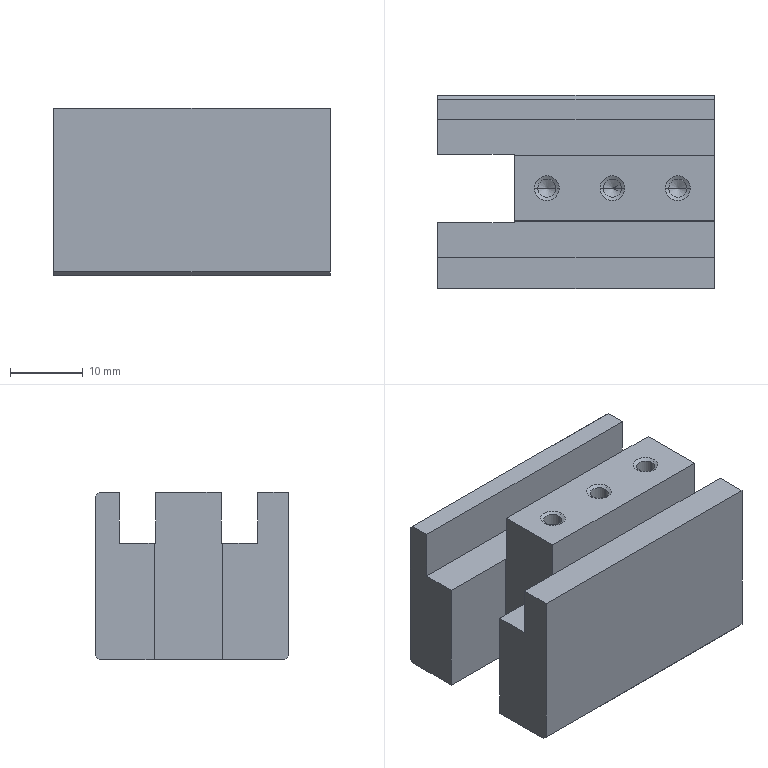Part | NX | 1 solid | 57 faces | box 38 x 26.5 x 22.95 mm | volume 17737 mm3 | cone 24 | plane 21 | cylinder 12 | commonest cylinder face diameters 2.5 x6 3.3 x6
STEP:
#1=CARTESIAN_POINT('',(0.,0.,-22.45));
#2=VERTEX_POINT('',#1);
#3=CARTESIAN_POINT('',(38.,0.,-22.45));
#4=VERTEX_POINT('',#3);
#5=CARTESIAN_POINT('',(0.,0.,-22.45));
#6=DIRECTION('',(1.,0.,0.));
#7=VECTOR('',#6,1000.);
#8=LINE('',#5,#7);
#9=EDGE_CURVE('',#2,#4,#8,.T.);
#10=ORIENTED_EDGE('',*,*,#9,.T.);
#11=CARTESIAN_POINT('',(38.,0.,0.));
#12=VERTEX_POINT('',#11);
#13=CARTESIAN_POINT('',(38.,0.,0.));
#14=DIRECTION('',(0.,0.,-1.));
#15=VECTOR('',#14,1000.);
#16=LINE('',#13,#15);
#17=EDGE_CURVE('',#12,#4,#16,.T.);
#18=ORIENTED_EDGE('',*,*,#17,.F.);
#19=CARTESIAN_POINT('',(0.,0.,0.));
#20=VERTEX_POINT('',#19);
#21=CARTESIAN_POINT('',(0.,0.,0.));
#22=DIRECTION('',(-1.,0.,0.));
#23=VECTOR('',#22,1000.);
#24=LINE('',#21,#23);
#25=EDGE_CURVE('',#12,#20,#24,.T.);
#26=ORIENTED_EDGE('',*,*,#25,.T.);
#27=CARTESIAN_POINT('',(0.,0.,0.));
#28=DIRECTION('',(0.,0.,1.));
#29=VECTOR('',#28,1000.);
#30=LINE('',#27,#29);
#31=EDGE_CURVE('',#2,#20,#30,.T.);
#32=ORIENTED_EDGE('',*,*,#31,.F.);
#33=EDGE_LOOP('',(#10,#18,#26,#32));
#34=FACE_BOUND('',#33,.T.);
#35=CARTESIAN_POINT('',(0.,0.,0.));
#36=DIRECTION('',(0.,1.,0.));
#37=DIRECTION('',(1.,0.,0.));
#38=AXIS2_PLACEMENT_3D('',#35,#36,#37);
#39=PLANE('',#38);
#40=ADVANCED_FACE('',(#34),#39,.F.);
#41=CARTESIAN_POINT('',(0.,4.25,0.));
#42=VERTEX_POINT('',#41);
#43=CARTESIAN_POINT('',(38.,4.25,0.));
#44=VERTEX_POINT('',#43);
#45=CARTESIAN_POINT('',(0.,4.25,0.));
#46=DIRECTION('',(1.,0.,0.));
#47=VECTOR('',#46,1000.);
#48=LINE('',#45,#47);
#49=EDGE_CURVE('',#42,#44,#48,.T.);
#50=ORIENTED_EDGE('',*,*,#49,.F.);
#51=CARTESIAN_POINT('',(0.,0.,0.));
#52=DIRECTION('',(0.,-1.,0.));
#53=VECTOR('',#52,1000.);
#54=LINE('',#51,#53);
#55=EDGE_CURVE('',#42,#20,#54,.T.);
#56=ORIENTED_EDGE('',*,*,#55,.T.);
#57=ORIENTED_EDGE('',*,*,#25,.F.);
#58=CARTESIAN_POINT('',(38.,0.,0.));
#59=DIRECTION('',(0.,1.,0.));
#60=VECTOR('',#59,1000.);
#61=LINE('',#58,#60);
#62=EDGE_CURVE('',#12,#44,#61,.T.);
#63=ORIENTED_EDGE('',*,*,#62,.T.);
#64=EDGE_LOOP('',(#50,#56,#57,#63));
#65=FACE_BOUND('',#64,.T.);
#66=CARTESIAN_POINT('',(0.,0.,0.));
#67=DIRECTION('',(0.,0.,1.));
#68=DIRECTION('',(1.,0.,0.));
#69=AXIS2_PLACEMENT_3D('',#66,#67,#68);
#70=PLANE('',#69);
#71=ADVANCED_FACE('',(#65),#70,.T.);
#72=ORIENTED_EDGE('',*,*,#49,.T.);
#73=CARTESIAN_POINT('',(38.,4.25,-7.));
#74=VERTEX_POINT('',#73);
#75=CARTESIAN_POINT('',(38.,4.25,0.));
#76=DIRECTION('',(0.,0.,1.));
#77=VECTOR('',#76,1000.);
#78=LINE('',#75,#77);
#79=EDGE_CURVE('',#74,#44,#78,.T.);
#80=ORIENTED_EDGE('',*,*,#79,.F.);
#81=CARTESIAN_POINT('',(0.,4.25,-7.));
#82=VERTEX_POINT('',#81);
#83=CARTESIAN_POINT('',(0.,4.25,-7.));
#84=DIRECTION('',(1.,0.,0.));
#85=VECTOR('',#84,1000.);
#86=LINE('',#83,#85);
#87=EDGE_CURVE('',#82,#74,#86,.T.);
#88=ORIENTED_EDGE('',*,*,#87,.F.);
#89=CARTESIAN_POINT('',(0.,4.25,0.));
#90=DIRECTION('',(0.,0.,-1.));
#91=VECTOR('',#90,1000.);
#92=LINE('',#89,#91);
#93=EDGE_CURVE('',#42,#82,#92,.T.);
#94=ORIENTED_EDGE('',*,*,#93,.F.);
#95=EDGE_LOOP('',(#72,#80,#88,#94));
#96=FACE_BOUND('',#95,.T.);
#97=CARTESIAN_POINT('',(0.,4.25,-7.));
#98=DIRECTION('',(0.,-1.,0.));
#99=DIRECTION('',(0.,0.,-1.));
#100=AXIS2_PLACEMENT_3D('',#97,#98,#99);
#101=PLANE('',#100);
#102=ADVANCED_FACE('',(#96),#101,.F.);
#103=CARTESIAN_POINT('',(0.,9.05,-22.95));
#104=VERTEX_POINT('',#103);
#105=CARTESIAN_POINT('',(0.,9.05,-7.));
#106=VERTEX_POINT('',#105);
#107=CARTESIAN_POINT('',(0.,9.05,0.));
#108=DIRECTION('',(0.,0.,1.));
#109=VECTOR('',#108,1000.);
#110=LINE('',#107,#109);
#111=EDGE_CURVE('',#104,#106,#110,.T.);
#112=ORIENTED_EDGE('',*,*,#111,.F.);
#113=CARTESIAN_POINT('',(0.,0.5,-22.95));
#114=VERTEX_POINT('',#113);
#115=CARTESIAN_POINT('',(0.,0.,-22.95));
#116=DIRECTION('',(0.,-1.,0.));
#117=VECTOR('',#116,1000.);
#118=LINE('',#115,#117);
#119=EDGE_CURVE('',#104,#114,#118,.T.);
#120=ORIENTED_EDGE('',*,*,#119,.T.);
#121=CARTESIAN_POINT('',(0.,-22.45,0.));
#122=DIRECTION('',(0.,-0.7071,0.7071));
#123=VECTOR('',#122,1000.);
#124=LINE('',#121,#123);
#125=EDGE_CURVE('',#114,#2,#124,.T.);
#126=ORIENTED_EDGE('',*,*,#125,.T.);
#127=ORIENTED_EDGE('',*,*,#31,.T.);
#128=ORIENTED_EDGE('',*,*,#55,.F.);
#129=ORIENTED_EDGE('',*,*,#93,.T.);
#130=CARTESIAN_POINT('',(0.,0.,-7.));
#131=DIRECTION('',(0.,-1.,0.));
#132=VECTOR('',#131,1000.);
#133=LINE('',#130,#132);
#134=EDGE_CURVE('',#106,#82,#133,.T.);
#135=ORIENTED_EDGE('',*,*,#134,.F.);
#136=EDGE_LOOP('',(#112,#120,#126,#127,#128,#129,#135));
#137=FACE_BOUND('',#136,.T.);
#138=CARTESIAN_POINT('',(0.,0.,-23.));
#139=DIRECTION('',(-1.,0.,0.));
#140=DIRECTION('',(0.,0.,1.));
#141=AXIS2_PLACEMENT_3D('',#138,#139,#140);
#142=PLANE('',#141);
#143=ADVANCED_FACE('',(#137),#142,.T.);
#144=CARTESIAN_POINT('',(10.5,9.05,-22.95));
#145=VERTEX_POINT('',#144);
#146=CARTESIAN_POINT('',(0.,9.05,-22.95));
#147=DIRECTION('',(1.,0.,0.));
#148=VECTOR('',#147,1000.);
#149=LINE('',#146,#148);
#150=EDGE_CURVE('',#104,#145,#149,.T.);
#151=ORIENTED_EDGE('',*,*,#150,.F.);
#152=ORIENTED_EDGE('',*,*,#111,.T.);
#153=CARTESIAN_POINT('',(10.5,9.05,-7.));
#154=VERTEX_POINT('',#153);
#155=CARTESIAN_POINT('',(0.,9.05,-7.));
#156=DIRECTION('',(-1.,0.,0.));
#157=VECTOR('',#156,1000.);
#158=LINE('',#155,#157);
#159=EDGE_CURVE('',#154,#106,#158,.T.);
#160=ORIENTED_EDGE('',*,*,#159,.F.);
#161=CARTESIAN_POINT('',(10.5,9.05,0.));
#162=DIRECTION('',(0.,0.,1.));
#163=VECTOR('',#162,1000.);
#164=LINE('',#161,#163);
#165=EDGE_CURVE('',#145,#154,#164,.T.);
#166=ORIENTED_EDGE('',*,*,#165,.F.);
#167=EDGE_LOOP('',(#151,#152,#160,#166));
#168=FACE_BOUND('',#167,.T.);
#169=CARTESIAN_POINT('',(10.,9.05,-23.));
#170=DIRECTION('',(0.,-1.,0.));
#171=DIRECTION('',(0.,0.,-1.));
#172=AXIS2_PLACEMENT_3D('',#169,#170,#171);
#173=PLANE('',#172);
#174=ADVANCED_FACE('',(#168),#173,.F.);
#175=CARTESIAN_POINT('',(13.75,13.75,-9.));
#176=VERTEX_POINT('',#175);
#177=CARTESIAN_POINT('',(16.25,13.75,-9.));
#178=VERTEX_POINT('',#177);
#179=CARTESIAN_POINT('',(15.,13.75,-9.));
#180=DIRECTION('',(0.,0.,1.));
#181=DIRECTION('',(1.,0.,0.));
#182=AXIS2_PLACEMENT_3D('',#179,#180,#181);
#183=CIRCLE('',#182,1.25);
#184=EDGE_CURVE('',#176,#178,#183,.T.);
#185=ORIENTED_EDGE('',*,*,#184,.T.);
#186=CARTESIAN_POINT('',(15.,13.75,-9.751));
#187=VERTEX_POINT('',#186);
#188=CARTESIAN_POINT('',(16.25,13.75,-9.));
#189=DIRECTION('',(0.8572,0.,0.515));
#190=VECTOR('',#189,1000.);
#191=LINE('',#188,#190);
#192=EDGE_CURVE('',#178,#187,#191,.F.);
#193=ORIENTED_EDGE('',*,*,#192,.T.);
#194=CARTESIAN_POINT('',(13.75,13.75,-9.));
#195=DIRECTION('',(-0.8572,0.,0.515));
#196=VECTOR('',#195,1000.);
#197=LINE('',#194,#196);
#198=EDGE_CURVE('',#176,#187,#197,.F.);
#199=ORIENTED_EDGE('',*,*,#198,.F.);
#200=EDGE_LOOP('',(#185,#193,#199));
#201=FACE_BOUND('',#200,.T.);
#202=CARTESIAN_POINT('',(15.,13.75,-9.));
#203=DIRECTION('',(0.,0.,1.));
#204=DIRECTION('',(1.,0.,0.));
#205=AXIS2_PLACEMENT_3D('',#202,#203,#204);
#206=CONICAL_SURFACE('',#205,1.25,1.03);
#207=ADVANCED_FACE('',(#201),#206,.F.);
#208=CARTESIAN_POINT('',(10.5,18.45,-22.95));
#209=VERTEX_POINT('',#208);
#210=CARTESIAN_POINT('',(0.,18.45,-22.95));
#211=VERTEX_POINT('',#210);
#212=CARTESIAN_POINT('',(0.,18.45,-22.95));
#213=DIRECTION('',(-1.,0.,0.));
#214=VECTOR('',#213,1000.);
#215=LINE('',#212,#214);
#216=EDGE_CURVE('',#209,#211,#215,.T.);
#217=ORIENTED_EDGE('',*,*,#216,.F.);
#218=CARTESIAN_POINT('',(10.5,18.45,-7.));
#219=VERTEX_POINT('',#218);
#220=CARTESIAN_POINT('',(10.5,18.45,0.));
#221=DIRECTION('',(0.,0.,-1.));
#222=VECTOR('',#221,1000.);
#223=LINE('',#220,#222);
#224=EDGE_CURVE('',#219,#209,#223,.T.);
#225=ORIENTED_EDGE('',*,*,#224,.F.);
#226=CARTESIAN_POINT('',(0.,18.45,-7.));
#227=VERTEX_POINT('',#226);
#228=CARTESIAN_POINT('',(0.,18.45,-7.));
#229=DIRECTION('',(1.,0.,0.));
#230=VECTOR('',#229,1000.);
#231=LINE('',#228,#230);
#232=EDGE_CURVE('',#227,#219,#231,.T.);
#233=ORIENTED_EDGE('',*,*,#232,.F.);
#234=CARTESIAN_POINT('',(0.,18.45,0.));
#235=DIRECTION('',(0.,0.,-1.));
#236=VECTOR('',#235,1000.);
#237=LINE('',#234,#236);
#238=EDGE_CURVE('',#227,#211,#237,.T.);
#239=ORIENTED_EDGE('',*,*,#238,.T.);
#240=EDGE_LOOP('',(#217,#225,#233,#239));
#241=FACE_BOUND('',#240,.T.);
#242=CARTESIAN_POINT('',(0.,18.45,-23.));
#243=DIRECTION('',(0.,1.,0.));
#244=DIRECTION('',(1.,0.,0.));
#245=AXIS2_PLACEMENT_3D('',#242,#243,#244);
#246=PLANE('',#245);
#247=ADVANCED_FACE('',(#241),#246,.F.);
#248=ORIENTED_EDGE('',*,*,#238,.F.);
#249=CARTESIAN_POINT('',(0.,23.25,-7.));
#250=VERTEX_POINT('',#249);
#251=CARTESIAN_POINT('',(0.,0.,-7.));
#252=DIRECTION('',(0.,-1.,0.));
#253=VECTOR('',#252,1000.);
#254=LINE('',#251,#253);
#255=EDGE_CURVE('',#250,#227,#254,.T.);
#256=ORIENTED_EDGE('',*,*,#255,.F.);
#257=CARTESIAN_POINT('',(0.,23.25,0.));
#258=VERTEX_POINT('',#257);
#259=CARTESIAN_POINT('',(0.,23.25,0.));
#260=DIRECTION('',(0.,0.,1.));
#261=VECTOR('',#260,1000.);
#262=LINE('',#259,#261);
#263=EDGE_CURVE('',#250,#258,#262,.T.);
#264=ORIENTED_EDGE('',*,*,#263,.T.);
#265=CARTESIAN_POINT('',(0.,26.,0.));
#266=VERTEX_POINT('',#265);
#267=CARTESIAN_POINT('',(0.,0.,0.));
#268=DIRECTION('',(0.,-1.,0.));
#269=VECTOR('',#268,1000.);
#270=LINE('',#267,#269);
#271=EDGE_CURVE('',#266,#258,#270,.T.);
#272=ORIENTED_EDGE('',*,*,#271,.F.);
#273=CARTESIAN_POINT('',(0.,26.5,-0.5));
#274=VERTEX_POINT('',#273);
#275=CARTESIAN_POINT('',(0.,26.,0.));
#276=DIRECTION('',(0.,0.7071,-0.7071));
#277=VECTOR('',#276,1000.);
#278=LINE('',#275,#277);
#279=EDGE_CURVE('',#266,#274,#278,.T.);
#280=ORIENTED_EDGE('',*,*,#279,.T.);
#281=CARTESIAN_POINT('',(0.,26.5,-22.45));
#282=VERTEX_POINT('',#281);
#283=CARTESIAN_POINT('',(0.,26.5,0.));
#284=DIRECTION('',(0.,0.,1.));
#285=VECTOR('',#284,1000.);
#286=LINE('',#283,#285);
#287=EDGE_CURVE('',#282,#274,#286,.T.);
#288=ORIENTED_EDGE('',*,*,#287,.F.);
#289=CARTESIAN_POINT('',(0.,26.,-22.95));
#290=VERTEX_POINT('',#289);
#291=CARTESIAN_POINT('',(0.,48.95,0.));
#292=DIRECTION('',(0.,-0.7071,-0.7071));
#293=VECTOR('',#292,1000.);
#294=LINE('',#291,#293);
#295=EDGE_CURVE('',#282,#290,#294,.T.);
#296=ORIENTED_EDGE('',*,*,#295,.T.);
#297=CARTESIAN_POINT('',(0.,0.,-22.95));
#298=DIRECTION('',(0.,-1.,0.));
#299=VECTOR('',#298,1000.);
#300=LINE('',#297,#299);
#301=EDGE_CURVE('',#290,#211,#300,.T.);
#302=ORIENTED_EDGE('',*,*,#301,.T.);
#303=EDGE_LOOP('',(#248,#256,#264,#272,#280,#288,#296,#302));
#304=FACE_BOUND('',#303,.T.);
#305=CARTESIAN_POINT('',(0.,0.,-23.));
#306=DIRECTION('',(-1.,0.,0.));
#307=DIRECTION('',(0.,0.,1.));
#308=AXIS2_PLACEMENT_3D('',#305,#306,#307);
#309=PLANE('',#308);
#310=ADVANCED_FACE('',(#304),#309,.T.);
#311=CARTESIAN_POINT('',(38.,26.5,-0.5));
#312=VERTEX_POINT('',#311);
#313=CARTESIAN_POINT('',(0.,26.5,-0.5));
#314=DIRECTION('',(1.,0.,0.));
#315=VECTOR('',#314,1000.);
#316=LINE('',#313,#315);
#317=EDGE_CURVE('',#274,#312,#316,.T.);
#318=ORIENTED_EDGE('',*,*,#317,.T.);
#319=CARTESIAN_POINT('',(38.,26.5,-22.45));
#320=VERTEX_POINT('',#319);
#321=CARTESIAN_POINT('',(38.,26.5,0.));
#322=DIRECTION('',(0.,0.,1.));
#323=VECTOR('',#322,1000.);
#324=LINE('',#321,#323);
#325=EDGE_CURVE('',#320,#312,#324,.T.);
#326=ORIENTED_EDGE('',*,*,#325,.F.);
#327=CARTESIAN_POINT('',(0.,26.5,-22.45));
#328=DIRECTION('',(-1.,0.,0.));
#329=VECTOR('',#328,1000.);
#330=LINE('',#327,#329);
#331=EDGE_CURVE('',#320,#282,#330,.T.);
#332=ORIENTED_EDGE('',*,*,#331,.T.);
#333=ORIENTED_EDGE('',*,*,#287,.T.);
#334=EDGE_LOOP('',(#318,#326,#332,#333));
#335=FACE_BOUND('',#334,.T.);
#336=CARTESIAN_POINT('',(0.,26.5,0.));
#337=DIRECTION('',(0.,1.,0.));
#338=DIRECTION('',(1.,0.,0.));
#339=AXIS2_PLACEMENT_3D('',#336,#337,#338);
#340=PLANE('',#339);
#341=ADVANCED_FACE('',(#335),#340,.T.);
#342=CARTESIAN_POINT('',(38.,23.25,0.));
#343=VERTEX_POINT('',#342);
#344=CARTESIAN_POINT('',(0.,23.25,0.));
#345=DIRECTION('',(-1.,0.,0.));
#346=VECTOR('',#345,1000.);
#347=LINE('',#344,#346);
#348=EDGE_CURVE('',#343,#258,#347,.T.);
#349=ORIENTED_EDGE('',*,*,#348,.F.);
#350=CARTESIAN_POINT('',(38.,26.,0.));
#351=VERTEX_POINT('',#350);
#352=CARTESIAN_POINT('',(38.,0.,0.));
#353=DIRECTION('',(0.,1.,0.));
#354=VECTOR('',#353,1000.);
#355=LINE('',#352,#354);
#356=EDGE_CURVE('',#343,#351,#355,.T.);
#357=ORIENTED_EDGE('',*,*,#356,.T.);
#358=CARTESIAN_POINT('',(0.,26.,0.));
#359=DIRECTION('',(-1.,0.,0.));
#360=VECTOR('',#359,1000.);
#361=LINE('',#358,#360);
#362=EDGE_CURVE('',#351,#266,#361,.T.);
#363=ORIENTED_EDGE('',*,*,#362,.T.);
#364=ORIENTED_EDGE('',*,*,#271,.T.);
#365=EDGE_LOOP('',(#349,#357,#363,#364));
#366=FACE_BOUND('',#365,.T.);
#367=CARTESIAN_POINT('',(0.,0.,0.));
#368=DIRECTION('',(0.,0.,1.));
#369=DIRECTION('',(1.,0.,0.));
#370=AXIS2_PLACEMENT_3D('',#367,#368,#369);
#371=PLANE('',#370);
#372=ADVANCED_FACE('',(#366),#371,.T.);
#373=ORIENTED_EDGE('',*,*,#348,.T.);
#374=ORIENTED_EDGE('',*,*,#263,.F.);
#375=CARTESIAN_POINT('',(38.,23.25,-7.));
#376=VERTEX_POINT('',#375);
#377=CARTESIAN_POINT('',(0.,23.25,-7.));
#378=DIRECTION('',(-1.,0.,0.));
#379=VECTOR('',#378,1000.);
#380=LINE('',#377,#379);
#381=EDGE_CURVE('',#376,#250,#380,.T.);
#382=ORIENTED_EDGE('',*,*,#381,.F.);
#383=CARTESIAN_POINT('',(38.,23.25,0.));
#384=DIRECTION('',(0.,0.,-1.));
#385=VECTOR('',#384,1000.);
#386=LINE('',#383,#385);
#387=EDGE_CURVE('',#343,#376,#386,.T.);
#388=ORIENTED_EDGE('',*,*,#387,.F.);
#389=EDGE_LOOP('',(#373,#374,#382,#388));
#390=FACE_BOUND('',#389,.T.);
#391=CARTESIAN_POINT('',(0.,23.25,0.));
#392=DIRECTION('',(0.,1.,0.));
#393=DIRECTION('',(1.,0.,0.));
#394=AXIS2_PLACEMENT_3D('',#391,#392,#393);
#395=PLANE('',#394);
#396=ADVANCED_FACE('',(#390),#395,.F.);
#397=ORIENTED_EDGE('',*,*,#387,.T.);
#398=CARTESIAN_POINT('',(38.,18.25,-7.));
#399=VERTEX_POINT('',#398);
#400=CARTESIAN_POINT('',(38.,0.,-7.));
#401=DIRECTION('',(0.,1.,0.));
#402=VECTOR('',#401,1000.);
#403=LINE('',#400,#402);
#404=EDGE_CURVE('',#399,#376,#403,.T.);
#405=ORIENTED_EDGE('',*,*,#404,.F.);
#406=CARTESIAN_POINT('',(38.,18.25,0.));
#407=VERTEX_POINT('',#406);
#408=CARTESIAN_POINT('',(38.,18.25,0.));
#409=DIRECTION('',(0.,0.,-1.));
#410=VECTOR('',#409,1000.);
#411=LINE('',#408,#410);
#412=EDGE_CURVE('',#407,#399,#411,.T.);
#413=ORIENTED_EDGE('',*,*,#412,.F.);
#414=CARTESIAN_POINT('',(38.,9.25,0.));
#415=VERTEX_POINT('',#414);
#416=CARTESIAN_POINT('',(38.,0.,0.));
#417=DIRECTION('',(0.,-1.,0.));
#418=VECTOR('',#417,1000.);
#419=LINE('',#416,#418);
#420=EDGE_CURVE('',#407,#415,#419,.T.);
#421=ORIENTED_EDGE('',*,*,#420,.T.);
#422=CARTESIAN_POINT('',(38.,9.25,-7.));
#423=VERTEX_POINT('',#422);
#424=CARTESIAN_POINT('',(38.,9.25,0.));
#425=DIRECTION('',(0.,0.,1.));
#426=VECTOR('',#425,1000.);
#427=LINE('',#424,#426);
#428=EDGE_CURVE('',#423,#415,#427,.T.);
#429=ORIENTED_EDGE('',*,*,#428,.F.);
#430=CARTESIAN_POINT('',(38.,0.,-7.));
#431=DIRECTION('',(0.,1.,0.));
#432=VECTOR('',#431,1000.);
#433=LINE('',#430,#432);
#434=EDGE_CURVE('',#74,#423,#433,.T.);
#435=ORIENTED_EDGE('',*,*,#434,.F.);
#436=ORIENTED_EDGE('',*,*,#79,.T.);
#437=ORIENTED_EDGE('',*,*,#62,.F.);
#438=ORIENTED_EDGE('',*,*,#17,.T.);
#439=CARTESIAN_POINT('',(38.,0.5,-22.95));
#440=VERTEX_POINT('',#439);
#441=CARTESIAN_POINT('',(38.,-22.45,0.));
#442=DIRECTION('',(0.,-0.7071,0.7071));
#443=VECTOR('',#442,1000.);
#444=LINE('',#441,#443);
#445=EDGE_CURVE('',#440,#4,#444,.T.);
#446=ORIENTED_EDGE('',*,*,#445,.F.);
#447=CARTESIAN_POINT('',(38.,26.,-22.95));
#448=VERTEX_POINT('',#447);
#449=CARTESIAN_POINT('',(38.,0.,-22.95));
#450=DIRECTION('',(0.,1.,0.));
#451=VECTOR('',#450,1000.);
#452=LINE('',#449,#451);
#453=EDGE_CURVE('',#440,#448,#452,.T.);
#454=ORIENTED_EDGE('',*,*,#453,.T.);
#455=CARTESIAN_POINT('',(38.,48.95,0.));
#456=DIRECTION('',(0.,-0.7071,-0.7071));
#457=VECTOR('',#456,1000.);
#458=LINE('',#455,#457);
#459=EDGE_CURVE('',#320,#448,#458,.T.);
#460=ORIENTED_EDGE('',*,*,#459,.F.);
#461=ORIENTED_EDGE('',*,*,#325,.T.);
#462=CARTESIAN_POINT('',(38.,26.,0.));
#463=DIRECTION('',(0.,-0.7071,0.7071));
#464=VECTOR('',#463,1000.);
#465=LINE('',#462,#464);
#466=EDGE_CURVE('',#312,#351,#465,.T.);
#467=ORIENTED_EDGE('',*,*,#466,.T.);
#468=ORIENTED_EDGE('',*,*,#356,.F.);
#469=EDGE_LOOP('',(#397,#405,#413,#421,#429,#435,#436,#437,#438,#446,#454,#460,#461,#467,#468));
#470=FACE_BOUND('',#469,.T.);
#471=CARTESIAN_POINT('',(38.,0.,0.));
#472=DIRECTION('',(1.,0.,0.));
#473=DIRECTION('',(0.,1.,0.));
#474=AXIS2_PLACEMENT_3D('',#471,#472,#473);
#475=PLANE('',#474);
#476=ADVANCED_FACE('',(#470),#475,.T.);
#477=CARTESIAN_POINT('',(10.5,9.25,-7.));
#478=VERTEX_POINT('',#477);
#479=CARTESIAN_POINT('',(10.5,0.,-7.));
#480=DIRECTION('',(0.,-1.,0.));
#481=VECTOR('',#480,1000.);
#482=LINE('',#479,#481);
#483=EDGE_CURVE('',#478,#154,#482,.T.);
#484=ORIENTED_EDGE('',*,*,#483,.T.);
#485=ORIENTED_EDGE('',*,*,#159,.T.);
#486=ORIENTED_EDGE('',*,*,#134,.T.);
#487=ORIENTED_EDGE('',*,*,#87,.T.);
#488=ORIENTED_EDGE('',*,*,#434,.T.);
#489=CARTESIAN_POINT('',(0.,9.25,-7.));
#490=DIRECTION('',(1.,0.,0.));
#491=VECTOR('',#490,1000.);
#492=LINE('',#489,#491);
#493=EDGE_CURVE('',#478,#423,#492,.T.);
#494=ORIENTED_EDGE('',*,*,#493,.F.);
#495=EDGE_LOOP('',(#484,#485,#486,#487,#488,#494));
#496=FACE_BOUND('',#495,.T.);
#497=CARTESIAN_POINT('',(0.,9.25,-7.));
#498=DIRECTION('',(0.,0.,-1.));
#499=DIRECTION('',(0.,-1.,0.));
#500=AXIS2_PLACEMENT_3D('',#497,#498,#499);
#501=PLANE('',#500);
#502=ADVANCED_FACE('',(#496),#501,.F.);
#503=CARTESIAN_POINT('',(10.5,18.25,0.));
#504=VERTEX_POINT('',#503);
#505=CARTESIAN_POINT('',(10.5,9.25,0.));
#506=VERTEX_POINT('',#505);
#507=CARTESIAN_POINT('',(10.5,0.,0.));
#508=DIRECTION('',(0.,-1.,0.));
#509=VECTOR('',#508,1000.);
#510=LINE('',#507,#509);
#511=EDGE_CURVE('',#504,#506,#510,.T.);
#512=ORIENTED_EDGE('',*,*,#511,.F.);
#513=CARTESIAN_POINT('',(10.5,18.25,-7.));
#514=VERTEX_POINT('',#513);
#515=CARTESIAN_POINT('',(10.5,18.25,0.));
#516=DIRECTION('',(0.,0.,1.));
#517=VECTOR('',#516,1000.);
#518=LINE('',#515,#517);
#519=EDGE_CURVE('',#514,#504,#518,.T.);
#520=ORIENTED_EDGE('',*,*,#519,.F.);
#521=CARTESIAN_POINT('',(10.5,0.,-7.));
#522=DIRECTION('',(0.,-1.,0.));
#523=VECTOR('',#522,1000.);
#524=LINE('',#521,#523);
#525=EDGE_CURVE('',#219,#514,#524,.T.);
#526=ORIENTED_EDGE('',*,*,#525,.F.);
#527=ORIENTED_EDGE('',*,*,#224,.T.);
#528=CARTESIAN_POINT('',(10.5,0.,-22.95));
#529=DIRECTION('',(0.,1.,0.));
#530=VECTOR('',#529,1000.);
#531=LINE('',#528,#530);
#532=EDGE_CURVE('',#145,#209,#531,.T.);
#533=ORIENTED_EDGE('',*,*,#532,.F.);
#534=ORIENTED_EDGE('',*,*,#165,.T.);
#535=ORIENTED_EDGE('',*,*,#483,.F.);
#536=CARTESIAN_POINT('',(10.5,9.25,0.));
#537=DIRECTION('',(0.,0.,-1.));
#538=VECTOR('',#537,1000.);
#539=LINE('',#536,#538);
#540=EDGE_CURVE('',#506,#478,#539,.T.);
#541=ORIENTED_EDGE('',*,*,#540,.F.);
#542=EDGE_LOOP('',(#512,#520,#526,#527,#533,#534,#535,#541));
#543=FACE_BOUND('',#542,.T.);
#544=CARTESIAN_POINT('',(10.5,18.45,-23.));
#545=DIRECTION('',(1.,0.,0.));
#546=DIRECTION('',(0.,1.,0.));
#547=AXIS2_PLACEMENT_3D('',#544,#545,#546);
#548=PLANE('',#547);
#549=ADVANCED_FACE('',(#543),#548,.F.);
#550=CARTESIAN_POINT('',(0.,26.,-22.95));
#551=DIRECTION('',(1.,0.,0.));
#552=VECTOR('',#551,1000.);
#553=LINE('',#550,#552);
#554=EDGE_CURVE('',#290,#448,#553,.T.);
#555=ORIENTED_EDGE('',*,*,#554,.T.);
#556=ORIENTED_EDGE('',*,*,#453,.F.);
#557=CARTESIAN_POINT('',(0.,0.5,-22.95));
#558=DIRECTION('',(-1.,0.,0.));
#559=VECTOR('',#558,1000.);
#560=LINE('',#557,#559);
#561=EDGE_CURVE('',#440,#114,#560,.T.);
#562=ORIENTED_EDGE('',*,*,#561,.T.);
#563=ORIENTED_EDGE('',*,*,#119,.F.);
#564=ORIENTED_EDGE('',*,*,#150,.T.);
#565=ORIENTED_EDGE('',*,*,#532,.T.);
#566=ORIENTED_EDGE('',*,*,#216,.T.);
#567=ORIENTED_EDGE('',*,*,#301,.F.);
#568=EDGE_LOOP('',(#555,#556,#562,#563,#564,#565,#566,#567));
#569=FACE_BOUND('',#568,.T.);
#570=CARTESIAN_POINT('',(30.685,21.75,-22.95));
#571=VERTEX_POINT('',#570);
#572=CARTESIAN_POINT('',(35.315,21.75,-22.95));
#573=VERTEX_POINT('',#572);
#574=CARTESIAN_POINT('',(33.,21.75,-22.95));
#575=DIRECTION('',(0.,0.,-1.));
#576=DIRECTION('',(-1.,0.,0.));
#577=AXIS2_PLACEMENT_3D('',#574,#575,#576);
#578=CIRCLE('',#577,2.315);
#579=EDGE_CURVE('',#571,#573,#578,.T.);
#580=ORIENTED_EDGE('',*,*,#579,.F.);
#581=CARTESIAN_POINT('',(33.,21.75,-22.95));
#582=DIRECTION('',(0.,0.,-1.));
#583=DIRECTION('',(-1.,0.,0.));
#584=AXIS2_PLACEMENT_3D('',#581,#582,#583);
#585=CIRCLE('',#584,2.315);
#586=EDGE_CURVE('',#573,#571,#585,.T.);
#587=ORIENTED_EDGE('',*,*,#586,.F.);
#588=EDGE_LOOP('',(#580,#587));
#589=FACE_BOUND('',#588,.T.);
#590=CARTESIAN_POINT('',(7.315,21.75,-22.95));
#591=VERTEX_POINT('',#590);
#592=CARTESIAN_POINT('',(2.685,21.75,-22.95));
#593=VERTEX_POINT('',#592);
#594=CARTESIAN_POINT('',(5.,21.75,-22.95));
#595=DIRECTION('',(0.,0.,-1.));
#596=DIRECTION('',(-1.,0.,0.));
#597=AXIS2_PLACEMENT_3D('',#594,#595,#596);
#598=CIRCLE('',#597,2.315);
#599=EDGE_CURVE('',#591,#593,#598,.T.);
#600=ORIENTED_EDGE('',*,*,#599,.F.);
#601=CARTESIAN_POINT('',(5.,21.75,-22.95));
#602=DIRECTION('',(0.,0.,-1.));
#603=DIRECTION('',(-1.,0.,0.));
#604=AXIS2_PLACEMENT_3D('',#601,#602,#603);
#605=CIRCLE('',#604,2.315);
#606=EDGE_CURVE('',#593,#591,#605,.T.);
#607=ORIENTED_EDGE('',*,*,#606,.F.);
#608=EDGE_LOOP('',(#600,#607));
#609=FACE_BOUND('',#608,.T.);
#610=CARTESIAN_POINT('',(16.685,21.75,-22.95));
#611=VERTEX_POINT('',#610);
#612=CARTESIAN_POINT('',(21.315,21.75,-22.95));
#613=VERTEX_POINT('',#612);
#614=CARTESIAN_POINT('',(19.,21.75,-22.95));
#615=DIRECTION('',(0.,0.,-1.));
#616=DIRECTION('',(-1.,0.,0.));
#617=AXIS2_PLACEMENT_3D('',#614,#615,#616);
#618=CIRCLE('',#617,2.315);
#619=EDGE_CURVE('',#611,#613,#618,.T.);
#620=ORIENTED_EDGE('',*,*,#619,.F.);
#621=CARTESIAN_POINT('',(19.,21.75,-22.95));
#622=DIRECTION('',(0.,0.,-1.));
#623=DIRECTION('',(-1.,0.,0.));
#624=AXIS2_PLACEMENT_3D('',#621,#622,#623);
#625=CIRCLE('',#624,2.315);
#626=EDGE_CURVE('',#613,#611,#625,.T.);
#627=ORIENTED_EDGE('',*,*,#626,.F.);
#628=EDGE_LOOP('',(#620,#627));
#629=FACE_BOUND('',#628,.T.);
#630=CARTESIAN_POINT('',(38.,0.,-22.95));
#631=DIRECTION('',(0.,0.,-1.));
#632=DIRECTION('',(0.,-1.,0.));
#633=AXIS2_PLACEMENT_3D('',#630,#631,#632);
#634=PLANE('',#633);
#635=ADVANCED_FACE('',(#569,#589,#609,#629),#634,.T.);
#636=ORIENTED_EDGE('',*,*,#519,.T.);
#637=CARTESIAN_POINT('',(0.,18.25,0.));
#638=DIRECTION('',(-1.,0.,0.));
#639=VECTOR('',#638,1000.);
#640=LINE('',#637,#639);
#641=EDGE_CURVE('',#407,#504,#640,.T.);
#642=ORIENTED_EDGE('',*,*,#641,.F.);
#643=ORIENTED_EDGE('',*,*,#412,.T.);
#644=CARTESIAN_POINT('',(0.,18.25,-7.));
#645=DIRECTION('',(1.,0.,0.));
#646=VECTOR('',#645,1000.);
#647=LINE('',#644,#646);
#648=EDGE_CURVE('',#514,#399,#647,.T.);
#649=ORIENTED_EDGE('',*,*,#648,.F.);
#650=EDGE_LOOP('',(#636,#642,#643,#649));
#651=FACE_BOUND('',#650,.T.);
#652=CARTESIAN_POINT('',(0.,18.25,-7.));
#653=DIRECTION('',(0.,-1.,0.));
#654=DIRECTION('',(0.,0.,-1.));
#655=AXIS2_PLACEMENT_3D('',#652,#653,#654);
#656=PLANE('',#655);
#657=ADVANCED_FACE('',(#651),#656,.F.);
#658=ORIENTED_EDGE('',*,*,#232,.T.);
#659=ORIENTED_EDGE('',*,*,#525,.T.);
#660=ORIENTED_EDGE('',*,*,#648,.T.);
#661=ORIENTED_EDGE('',*,*,#404,.T.);
#662=ORIENTED_EDGE('',*,*,#381,.T.);
#663=ORIENTED_EDGE('',*,*,#255,.T.);
#664=EDGE_LOOP('',(#658,#659,#660,#661,#662,#663));
#665=FACE_BOUND('',#664,.T.);
#666=CARTESIAN_POINT('',(0.,23.25,-7.));
#667=DIRECTION('',(0.,0.,-1.));
#668=DIRECTION('',(0.,-1.,0.));
#669=AXIS2_PLACEMENT_3D('',#666,#667,#668);
#670=PLANE('',#669);
#671=ADVANCED_FACE('',(#665),#670,.F.);
#672=ORIENTED_EDGE('',*,*,#540,.T.);
#673=ORIENTED_EDGE('',*,*,#493,.T.);
#674=ORIENTED_EDGE('',*,*,#428,.T.);
#675=CARTESIAN_POINT('',(0.,9.25,0.));
#676=DIRECTION('',(1.,0.,0.));
#677=VECTOR('',#676,1000.);
#678=LINE('',#675,#677);
#679=EDGE_CURVE('',#506,#415,#678,.T.);
#680=ORIENTED_EDGE('',*,*,#679,.F.);
#681=EDGE_LOOP('',(#672,#673,#674,#680));
#682=FACE_BOUND('',#681,.T.);
#683=CARTESIAN_POINT('',(0.,9.25,0.));
#684=DIRECTION('',(0.,1.,0.));
#685=DIRECTION('',(1.,0.,0.));
#686=AXIS2_PLACEMENT_3D('',#683,#684,#685);
#687=PLANE('',#686);
#688=ADVANCED_FACE('',(#682),#687,.F.);
#689=CARTESIAN_POINT('',(34.25,13.75,-0.2598));
#690=VERTEX_POINT('',#689);
#691=CARTESIAN_POINT('',(31.75,13.75,-0.2598));
#692=VERTEX_POINT('',#691);
#693=CARTESIAN_POINT('',(33.,13.75,-0.2598));
#694=DIRECTION('',(0.,0.,1.));
#695=DIRECTION('',(1.,0.,0.));
#696=AXIS2_PLACEMENT_3D('',#693,#694,#695);
#697=CIRCLE('',#696,1.25);
#698=EDGE_CURVE('',#690,#692,#697,.T.);
#699=ORIENTED_EDGE('',*,*,#698,.F.);
#700=CARTESIAN_POINT('',(34.7,13.75,0.));
#701=VERTEX_POINT('',#700);
#702=CARTESIAN_POINT('',(34.25,13.75,-0.2598));
#703=DIRECTION('',(0.866,0.,0.5));
#704=VECTOR('',#703,1000.);
#705=LINE('',#702,#704);
#706=EDGE_CURVE('',#690,#701,#705,.T.);
#707=ORIENTED_EDGE('',*,*,#706,.T.);
#708=CARTESIAN_POINT('',(31.3,13.75,0.));
#709=VERTEX_POINT('',#708);
#710=CARTESIAN_POINT('',(33.,13.75,0.));
#711=DIRECTION('',(0.,0.,1.));
#712=DIRECTION('',(1.,0.,0.));
#713=AXIS2_PLACEMENT_3D('',#710,#711,#712);
#714=CIRCLE('',#713,1.7);
#715=EDGE_CURVE('',#701,#709,#714,.T.);
#716=ORIENTED_EDGE('',*,*,#715,.T.);
#717=CARTESIAN_POINT('',(31.75,13.75,-0.2598));
#718=DIRECTION('',(-0.866,0.,0.5));
#719=VECTOR('',#718,1000.);
#720=LINE('',#717,#719);
#721=EDGE_CURVE('',#692,#709,#720,.T.);
#722=ORIENTED_EDGE('',*,*,#721,.F.);
#723=EDGE_LOOP('',(#699,#707,#716,#722));
#724=FACE_BOUND('',#723,.T.);
#725=CARTESIAN_POINT('',(33.,13.75,-0.2598));
#726=DIRECTION('',(0.,0.,1.));
#727=DIRECTION('',(1.,0.,0.));
#728=AXIS2_PLACEMENT_3D('',#725,#726,#727);
#729=CONICAL_SURFACE('',#728,1.25,1.047);
#730=ADVANCED_FACE('',(#724),#729,.F.);
#731=CARTESIAN_POINT('',(25.25,13.75,-0.2598));
#732=VERTEX_POINT('',#731);
#733=CARTESIAN_POINT('',(22.75,13.75,-0.2598));
#734=VERTEX_POINT('',#733);
#735=CARTESIAN_POINT('',(24.,13.75,-0.2598));
#736=DIRECTION('',(0.,0.,1.));
#737=DIRECTION('',(1.,0.,0.));
#738=AXIS2_PLACEMENT_3D('',#735,#736,#737);
#739=CIRCLE('',#738,1.25);
#740=EDGE_CURVE('',#732,#734,#739,.T.);
#741=ORIENTED_EDGE('',*,*,#740,.T.);
#742=CARTESIAN_POINT('',(22.75,13.75,-9.));
#743=VERTEX_POINT('',#742);
#744=CARTESIAN_POINT('',(22.75,13.75,0.));
#745=DIRECTION('',(0.,0.,1.));
#746=VECTOR('',#745,1000.);
#747=LINE('',#744,#746);
#748=EDGE_CURVE('',#743,#734,#747,.T.);
#749=ORIENTED_EDGE('',*,*,#748,.F.);
#750=CARTESIAN_POINT('',(25.25,13.75,-9.));
#751=VERTEX_POINT('',#750);
#752=CARTESIAN_POINT('',(24.,13.75,-9.));
#753=DIRECTION('',(0.,0.,1.));
#754=DIRECTION('',(1.,0.,0.));
#755=AXIS2_PLACEMENT_3D('',#752,#753,#754);
#756=CIRCLE('',#755,1.25);
#757=EDGE_CURVE('',#751,#743,#756,.T.);
#758=ORIENTED_EDGE('',*,*,#757,.F.);
#759=CARTESIAN_POINT('',(25.25,13.75,0.));
#760=DIRECTION('',(0.,0.,1.));
#761=VECTOR('',#760,1000.);
#762=LINE('',#759,#761);
#763=EDGE_CURVE('',#751,#732,#762,.T.);
#764=ORIENTED_EDGE('',*,*,#763,.T.);
#765=EDGE_LOOP('',(#741,#749,#758,#764));
#766=FACE_BOUND('',#765,.T.);
#767=CARTESIAN_POINT('',(24.,13.75,0.));
#768=DIRECTION('',(0.,0.,1.));
#769=DIRECTION('',(1.,0.,0.));
#770=AXIS2_PLACEMENT_3D('',#767,#768,#769);
#771=CYLINDRICAL_SURFACE('',#770,1.25);
#772=ADVANCED_FACE('',(#766),#771,.F.);
#773=ORIENTED_EDGE('',*,*,#554,.F.);
#774=ORIENTED_EDGE('',*,*,#295,.F.);
#775=ORIENTED_EDGE('',*,*,#331,.F.);
#776=ORIENTED_EDGE('',*,*,#459,.T.);
#777=EDGE_LOOP('',(#773,#774,#775,#776));
#778=FACE_BOUND('',#777,.T.);
#779=CARTESIAN_POINT('',(19.,26.25,-22.7));
#780=DIRECTION('',(0.,-0.7071,0.7071));
#781=DIRECTION('',(-1.,0.,0.));
#782=AXIS2_PLACEMENT_3D('',#779,#780,#781);
#783=PLANE('',#782);
#784=ADVANCED_FACE('',(#778),#783,.F.);
#785=ORIENTED_EDGE('',*,*,#679,.T.);
#786=ORIENTED_EDGE('',*,*,#420,.F.);
#787=ORIENTED_EDGE('',*,*,#641,.T.);
#788=ORIENTED_EDGE('',*,*,#511,.T.);
#789=EDGE_LOOP('',(#785,#786,#787,#788));
#790=FACE_BOUND('',#789,.T.);
#791=CARTESIAN_POINT('',(33.,13.75,0.));
#792=DIRECTION('',(0.,0.,1.));
#793=DIRECTION('',(1.,0.,0.));
#794=AXIS2_PLACEMENT_3D('',#791,#792,#793);
#795=CIRCLE('',#794,1.7);
#796=EDGE_CURVE('',#709,#701,#795,.T.);
#797=ORIENTED_EDGE('',*,*,#796,.F.);
#798=ORIENTED_EDGE('',*,*,#715,.F.);
#799=EDGE_LOOP('',(#797,#798));
#800=FACE_BOUND('',#799,.T.);
#801=CARTESIAN_POINT('',(16.7,13.75,0.));
#802=VERTEX_POINT('',#801);
#803=CARTESIAN_POINT('',(13.3,13.75,0.));
#804=VERTEX_POINT('',#803);
#805=CARTESIAN_POINT('',(15.,13.75,0.));
#806=DIRECTION('',(0.,0.,1.));
#807=DIRECTION('',(1.,0.,0.));
#808=AXIS2_PLACEMENT_3D('',#805,#806,#807);
#809=CIRCLE('',#808,1.7);
#810=EDGE_CURVE('',#802,#804,#809,.T.);
#811=ORIENTED_EDGE('',*,*,#810,.F.);
#812=CARTESIAN_POINT('',(15.,13.75,0.));
#813=DIRECTION('',(0.,0.,1.));
#814=DIRECTION('',(1.,0.,0.));
#815=AXIS2_PLACEMENT_3D('',#812,#813,#814);
#816=CIRCLE('',#815,1.7);
#817=EDGE_CURVE('',#804,#802,#816,.T.);
#818=ORIENTED_EDGE('',*,*,#817,.F.);
#819=EDGE_LOOP('',(#811,#818));
#820=FACE_BOUND('',#819,.T.);
#821=CARTESIAN_POINT('',(22.3,13.75,0.));
#822=VERTEX_POINT('',#821);
#823=CARTESIAN_POINT('',(25.7,13.75,0.));
#824=VERTEX_POINT('',#823);
#825=CARTESIAN_POINT('',(24.,13.75,0.));
#826=DIRECTION('',(0.,0.,1.));
#827=DIRECTION('',(1.,0.,0.));
#828=AXIS2_PLACEMENT_3D('',#825,#826,#827);
#829=CIRCLE('',#828,1.7);
#830=EDGE_CURVE('',#822,#824,#829,.T.);
#831=ORIENTED_EDGE('',*,*,#830,.F.);
#832=CARTESIAN_POINT('',(24.,13.75,0.));
#833=DIRECTION('',(0.,0.,1.));
#834=DIRECTION('',(1.,0.,0.));
#835=AXIS2_PLACEMENT_3D('',#832,#833,#834);
#836=CIRCLE('',#835,1.7);
#837=EDGE_CURVE('',#824,#822,#836,.T.);
#838=ORIENTED_EDGE('',*,*,#837,.F.);
#839=EDGE_LOOP('',(#831,#838));
#840=FACE_BOUND('',#839,.T.);
#841=CARTESIAN_POINT('',(0.,2.75,0.));
#842=DIRECTION('',(0.,0.,1.));
#843=DIRECTION('',(1.,0.,0.));
#844=AXIS2_PLACEMENT_3D('',#841,#842,#843);
#845=PLANE('',#844);
#846=ADVANCED_FACE('',(#790,#800,#820,#840),#845,.T.);
#847=ORIENTED_EDGE('',*,*,#757,.T.);
#848=CARTESIAN_POINT('',(24.,13.75,-9.751));
#849=VERTEX_POINT('',#848);
#850=CARTESIAN_POINT('',(22.75,13.75,-9.));
#851=DIRECTION('',(-0.8572,0.,0.515));
#852=VECTOR('',#851,1000.);
#853=LINE('',#850,#852);
#854=EDGE_CURVE('',#743,#849,#853,.F.);
#855=ORIENTED_EDGE('',*,*,#854,.T.);
#856=CARTESIAN_POINT('',(25.25,13.75,-9.));
#857=DIRECTION('',(0.8572,0.,0.515));
#858=VECTOR('',#857,1000.);
#859=LINE('',#856,#858);
#860=EDGE_CURVE('',#751,#849,#859,.F.);
#861=ORIENTED_EDGE('',*,*,#860,.F.);
#862=EDGE_LOOP('',(#847,#855,#861));
#863=FACE_BOUND('',#862,.T.);
#864=CARTESIAN_POINT('',(24.,13.75,-9.));
#865=DIRECTION('',(0.,0.,1.));
#866=DIRECTION('',(1.,0.,0.));
#867=AXIS2_PLACEMENT_3D('',#864,#865,#866);
#868=CONICAL_SURFACE('',#867,1.25,1.03);
#869=ADVANCED_FACE('',(#863),#868,.F.);
#870=ORIENTED_EDGE('',*,*,#317,.F.);
#871=ORIENTED_EDGE('',*,*,#279,.F.);
#872=ORIENTED_EDGE('',*,*,#362,.F.);
#873=ORIENTED_EDGE('',*,*,#466,.F.);
#874=EDGE_LOOP('',(#870,#871,#872,#873));
#875=FACE_BOUND('',#874,.T.);
#876=CARTESIAN_POINT('',(19.,26.25,-0.25));
#877=DIRECTION('',(0.,-0.7071,-0.7071));
#878=DIRECTION('',(0.,-0.7071,0.7071));
#879=AXIS2_PLACEMENT_3D('',#876,#877,#878);
#880=PLANE('',#879);
#881=ADVANCED_FACE('',(#875),#880,.F.);
#882=ORIENTED_EDGE('',*,*,#184,.F.);
#883=CARTESIAN_POINT('',(13.75,13.75,-0.2598));
#884=VERTEX_POINT('',#883);
#885=CARTESIAN_POINT('',(13.75,13.75,0.));
#886=DIRECTION('',(0.,0.,1.));
#887=VECTOR('',#886,1000.);
#888=LINE('',#885,#887);
#889=EDGE_CURVE('',#176,#884,#888,.T.);
#890=ORIENTED_EDGE('',*,*,#889,.T.);
#891=CARTESIAN_POINT('',(16.25,13.75,-0.2598));
#892=VERTEX_POINT('',#891);
#893=CARTESIAN_POINT('',(15.,13.75,-0.2598));
#894=DIRECTION('',(0.,0.,1.));
#895=DIRECTION('',(1.,0.,0.));
#896=AXIS2_PLACEMENT_3D('',#893,#894,#895);
#897=CIRCLE('',#896,1.25);
#898=EDGE_CURVE('',#884,#892,#897,.T.);
#899=ORIENTED_EDGE('',*,*,#898,.T.);
#900=CARTESIAN_POINT('',(16.25,13.75,0.));
#901=DIRECTION('',(0.,0.,1.));
#902=VECTOR('',#901,1000.);
#903=LINE('',#900,#902);
#904=EDGE_CURVE('',#178,#892,#903,.T.);
#905=ORIENTED_EDGE('',*,*,#904,.F.);
#906=EDGE_LOOP('',(#882,#890,#899,#905));
#907=FACE_BOUND('',#906,.T.);
#908=CARTESIAN_POINT('',(15.,13.75,0.));
#909=DIRECTION('',(0.,0.,1.));
#910=DIRECTION('',(1.,0.,0.));
#911=AXIS2_PLACEMENT_3D('',#908,#909,#910);
#912=CYLINDRICAL_SURFACE('',#911,1.25);
#913=ADVANCED_FACE('',(#907),#912,.F.);
#914=CARTESIAN_POINT('',(3.35,21.75,-22.566));
#915=VERTEX_POINT('',#914);
#916=CARTESIAN_POINT('',(6.65,21.75,-22.566));
#917=VERTEX_POINT('',#916);
#918=CARTESIAN_POINT('',(5.,21.75,-22.566));
#919=DIRECTION('',(0.,0.,-1.));
#920=DIRECTION('',(-1.,0.,0.));
#921=AXIS2_PLACEMENT_3D('',#918,#919,#920);
#922=CIRCLE('',#921,1.65);
#923=EDGE_CURVE('',#915,#917,#922,.T.);
#924=ORIENTED_EDGE('',*,*,#923,.F.);
#925=CARTESIAN_POINT('',(3.35,21.75,-22.566));
#926=DIRECTION('',(-0.866,0.,-0.5));
#927=VECTOR('',#926,1000.);
#928=LINE('',#925,#927);
#929=EDGE_CURVE('',#593,#915,#928,.F.);
#930=ORIENTED_EDGE('',*,*,#929,.F.);
#931=ORIENTED_EDGE('',*,*,#606,.T.);
#932=CARTESIAN_POINT('',(6.65,21.75,-22.566));
#933=DIRECTION('',(0.866,0.,-0.5));
#934=VECTOR('',#933,1000.);
#935=LINE('',#932,#934);
#936=EDGE_CURVE('',#591,#917,#935,.F.);
#937=ORIENTED_EDGE('',*,*,#936,.T.);
#938=EDGE_LOOP('',(#924,#930,#931,#937));
#939=FACE_BOUND('',#938,.T.);
#940=CARTESIAN_POINT('',(5.,21.75,-22.566));
#941=DIRECTION('',(0.,0.,-1.));
#942=DIRECTION('',(-1.,0.,0.));
#943=AXIS2_PLACEMENT_3D('',#940,#941,#942);
#944=CONICAL_SURFACE('',#943,1.65,1.047);
#945=ADVANCED_FACE('',(#939),#944,.F.);
#946=CARTESIAN_POINT('',(6.65,21.75,-10.75));
#947=VERTEX_POINT('',#946);
#948=CARTESIAN_POINT('',(3.35,21.75,-10.75));
#949=VERTEX_POINT('',#948);
#950=CARTESIAN_POINT('',(5.,21.75,-10.75));
#951=DIRECTION('',(0.,0.,-1.));
#952=DIRECTION('',(-1.,0.,0.));
#953=AXIS2_PLACEMENT_3D('',#950,#951,#952);
#954=CIRCLE('',#953,1.65);
#955=EDGE_CURVE('',#947,#949,#954,.T.);
#956=ORIENTED_EDGE('',*,*,#955,.F.);
#957=CARTESIAN_POINT('',(6.65,21.75,-22.95));
#958=DIRECTION('',(0.,0.,-1.));
#959=VECTOR('',#958,1000.);
#960=LINE('',#957,#959);
#961=EDGE_CURVE('',#947,#917,#960,.T.);
#962=ORIENTED_EDGE('',*,*,#961,.T.);
#963=CARTESIAN_POINT('',(5.,21.75,-22.566));
#964=DIRECTION('',(0.,0.,-1.));
#965=DIRECTION('',(-1.,0.,0.));
#966=AXIS2_PLACEMENT_3D('',#963,#964,#965);
#967=CIRCLE('',#966,1.65);
#968=EDGE_CURVE('',#917,#915,#967,.T.);
#969=ORIENTED_EDGE('',*,*,#968,.T.);
#970=CARTESIAN_POINT('',(3.35,21.75,-22.95));
#971=DIRECTION('',(0.,0.,-1.));
#972=VECTOR('',#971,1000.);
#973=LINE('',#970,#972);
#974=EDGE_CURVE('',#949,#915,#973,.T.);
#975=ORIENTED_EDGE('',*,*,#974,.F.);
#976=EDGE_LOOP('',(#956,#962,#969,#975));
#977=FACE_BOUND('',#976,.T.);
#978=CARTESIAN_POINT('',(5.,21.75,-22.95));
#979=DIRECTION('',(0.,0.,-1.));
#980=DIRECTION('',(-1.,0.,0.));
#981=AXIS2_PLACEMENT_3D('',#978,#979,#980);
#982=CYLINDRICAL_SURFACE('',#981,1.65);
#983=ADVANCED_FACE('',(#977),#982,.F.);
#984=ORIENTED_EDGE('',*,*,#9,.F.);
#985=ORIENTED_EDGE('',*,*,#125,.F.);
#986=ORIENTED_EDGE('',*,*,#561,.F.);
#987=ORIENTED_EDGE('',*,*,#445,.T.);
#988=EDGE_LOOP('',(#984,#985,#986,#987));
#989=FACE_BOUND('',#988,.T.);
#990=CARTESIAN_POINT('',(19.,0.25,-22.7));
#991=DIRECTION('',(0.,0.7071,0.7071));
#992=DIRECTION('',(1.,0.,0.));
#993=AXIS2_PLACEMENT_3D('',#990,#991,#992);
#994=PLANE('',#993);
#995=ADVANCED_FACE('',(#989),#994,.F.);
#996=ORIENTED_EDGE('',*,*,#740,.F.);
#997=CARTESIAN_POINT('',(25.25,13.75,-0.2598));
#998=DIRECTION('',(0.866,0.,0.5));
#999=VECTOR('',#998,1000.);
#1000=LINE('',#997,#999);
#1001=EDGE_CURVE('',#732,#824,#1000,.T.);
#1002=ORIENTED_EDGE('',*,*,#1001,.T.);
#1003=ORIENTED_EDGE('',*,*,#837,.T.);
#1004=CARTESIAN_POINT('',(22.75,13.75,-0.2598));
#1005=DIRECTION('',(-0.866,0.,0.5));
#1006=VECTOR('',#1005,1000.);
#1007=LINE('',#1004,#1006);
#1008=EDGE_CURVE('',#734,#822,#1007,.T.);
#1009=ORIENTED_EDGE('',*,*,#1008,.F.);
#1010=EDGE_LOOP('',(#996,#1002,#1003,#1009));
#1011=FACE_BOUND('',#1010,.T.);
#1012=CARTESIAN_POINT('',(24.,13.75,-0.2598));
#1013=DIRECTION('',(0.,0.,1.));
#1014=DIRECTION('',(1.,0.,0.));
#1015=AXIS2_PLACEMENT_3D('',#1012,#1013,#1014);
#1016=CONICAL_SURFACE('',#1015,1.25,1.047);
#1017=ADVANCED_FACE('',(#1011),#1016,.F.);
#1018=ORIENTED_EDGE('',*,*,#810,.T.);
#1019=CARTESIAN_POINT('',(13.75,13.75,-0.2598));
#1020=DIRECTION('',(-0.866,0.,0.5));
#1021=VECTOR('',#1020,1000.);
#1022=LINE('',#1019,#1021);
#1023=EDGE_CURVE('',#804,#884,#1022,.F.);
#1024=ORIENTED_EDGE('',*,*,#1023,.T.);
#1025=CARTESIAN_POINT('',(15.,13.75,-0.2598));
#1026=DIRECTION('',(0.,0.,1.));
#1027=DIRECTION('',(1.,0.,0.));
#1028=AXIS2_PLACEMENT_3D('',#1025,#1026,#1027);
#1029=CIRCLE('',#1028,1.25);
#1030=EDGE_CURVE('',#892,#884,#1029,.T.);
#1031=ORIENTED_EDGE('',*,*,#1030,.F.);
#1032=CARTESIAN_POINT('',(16.25,13.75,-0.2598));
#1033=DIRECTION('',(0.866,0.,0.5));
#1034=VECTOR('',#1033,1000.);
#1035=LINE('',#1032,#1034);
#1036=EDGE_CURVE('',#802,#892,#1035,.F.);
#1037=ORIENTED_EDGE('',*,*,#1036,.F.);
#1038=EDGE_LOOP('',(#1018,#1024,#1031,#1037));
#1039=FACE_BOUND('',#1038,.T.);
#1040=CARTESIAN_POINT('',(15.,13.75,-0.2598));
#1041=DIRECTION('',(0.,0.,1.));
#1042=DIRECTION('',(1.,0.,0.));
#1043=AXIS2_PLACEMENT_3D('',#1040,#1041,#1042);
#1044=CONICAL_SURFACE('',#1043,1.25,1.047);
#1045=ADVANCED_FACE('',(#1039),#1044,.F.);
#1046=CARTESIAN_POINT('',(34.25,13.75,-9.));
#1047=VERTEX_POINT('',#1046);
#1048=CARTESIAN_POINT('',(31.75,13.75,-9.));
#1049=VERTEX_POINT('',#1048);
#1050=CARTESIAN_POINT('',(33.,13.75,-9.));
#1051=DIRECTION('',(0.,0.,1.));
#1052=DIRECTION('',(1.,0.,0.));
#1053=AXIS2_PLACEMENT_3D('',#1050,#1051,#1052);
#1054=CIRCLE('',#1053,1.25);
#1055=EDGE_CURVE('',#1047,#1049,#1054,.T.);
#1056=ORIENTED_EDGE('',*,*,#1055,.F.);
#1057=CARTESIAN_POINT('',(34.25,13.75,0.));
#1058=DIRECTION('',(0.,0.,1.));
#1059=VECTOR('',#1058,1000.);
#1060=LINE('',#1057,#1059);
#1061=EDGE_CURVE('',#1047,#690,#1060,.T.);
#1062=ORIENTED_EDGE('',*,*,#1061,.T.);
#1063=ORIENTED_EDGE('',*,*,#698,.T.);
#1064=CARTESIAN_POINT('',(31.75,13.75,0.));
#1065=DIRECTION('',(0.,0.,1.));
#1066=VECTOR('',#1065,1000.);
#1067=LINE('',#1064,#1066);
#1068=EDGE_CURVE('',#1049,#692,#1067,.T.);
#1069=ORIENTED_EDGE('',*,*,#1068,.F.);
#1070=EDGE_LOOP('',(#1056,#1062,#1063,#1069));
#1071=FACE_BOUND('',#1070,.T.);
#1072=CARTESIAN_POINT('',(33.,13.75,0.));
#1073=DIRECTION('',(0.,0.,1.));
#1074=DIRECTION('',(1.,0.,0.));
#1075=AXIS2_PLACEMENT_3D('',#1072,#1073,#1074);
#1076=CYLINDRICAL_SURFACE('',#1075,1.25);
#1077=ADVANCED_FACE('',(#1071),#1076,.F.);
#1078=ORIENTED_EDGE('',*,*,#619,.T.);
#1079=CARTESIAN_POINT('',(20.65,21.75,-22.566));
#1080=VERTEX_POINT('',#1079);
#1081=CARTESIAN_POINT('',(20.65,21.75,-22.566));
#1082=DIRECTION('',(0.866,0.,-0.5));
#1083=VECTOR('',#1082,1000.);
#1084=LINE('',#1081,#1083);
#1085=EDGE_CURVE('',#1080,#613,#1084,.T.);
#1086=ORIENTED_EDGE('',*,*,#1085,.F.);
#1087=CARTESIAN_POINT('',(17.35,21.75,-22.566));
#1088=VERTEX_POINT('',#1087);
#1089=CARTESIAN_POINT('',(19.,21.75,-22.566));
#1090=DIRECTION('',(0.,0.,-1.));
#1091=DIRECTION('',(-1.,0.,0.));
#1092=AXIS2_PLACEMENT_3D('',#1089,#1090,#1091);
#1093=CIRCLE('',#1092,1.65);
#1094=EDGE_CURVE('',#1088,#1080,#1093,.T.);
#1095=ORIENTED_EDGE('',*,*,#1094,.F.);
#1096=CARTESIAN_POINT('',(17.35,21.75,-22.566));
#1097=DIRECTION('',(-0.866,0.,-0.5));
#1098=VECTOR('',#1097,1000.);
#1099=LINE('',#1096,#1098);
#1100=EDGE_CURVE('',#1088,#611,#1099,.T.);
#1101=ORIENTED_EDGE('',*,*,#1100,.T.);
#1102=EDGE_LOOP('',(#1078,#1086,#1095,#1101));
#1103=FACE_BOUND('',#1102,.T.);
#1104=CARTESIAN_POINT('',(19.,21.75,-22.566));
#1105=DIRECTION('',(0.,0.,-1.));
#1106=DIRECTION('',(-1.,0.,0.));
#1107=AXIS2_PLACEMENT_3D('',#1104,#1105,#1106);
#1108=CONICAL_SURFACE('',#1107,1.65,1.047);
#1109=ADVANCED_FACE('',(#1103),#1108,.F.);
#1110=ORIENTED_EDGE('',*,*,#1055,.T.);
#1111=CARTESIAN_POINT('',(33.,13.75,-9.751));
#1112=VERTEX_POINT('',#1111);
#1113=CARTESIAN_POINT('',(31.75,13.75,-9.));
#1114=DIRECTION('',(-0.8572,0.,0.515));
#1115=VECTOR('',#1114,1000.);
#1116=LINE('',#1113,#1115);
#1117=EDGE_CURVE('',#1049,#1112,#1116,.F.);
#1118=ORIENTED_EDGE('',*,*,#1117,.T.);
#1119=CARTESIAN_POINT('',(34.25,13.75,-9.));
#1120=DIRECTION('',(0.8572,0.,0.515));
#1121=VECTOR('',#1120,1000.);
#1122=LINE('',#1119,#1121);
#1123=EDGE_CURVE('',#1047,#1112,#1122,.F.);
#1124=ORIENTED_EDGE('',*,*,#1123,.F.);
#1125=EDGE_LOOP('',(#1110,#1118,#1124));
#1126=FACE_BOUND('',#1125,.T.);
#1127=CARTESIAN_POINT('',(33.,13.75,-9.));
#1128=DIRECTION('',(0.,0.,1.));
#1129=DIRECTION('',(1.,0.,0.));
#1130=AXIS2_PLACEMENT_3D('',#1127,#1128,#1129);
#1131=CONICAL_SURFACE('',#1130,1.25,1.03);
#1132=ADVANCED_FACE('',(#1126),#1131,.F.);
#1133=CARTESIAN_POINT('',(31.35,21.75,-22.566));
#1134=VERTEX_POINT('',#1133);
#1135=CARTESIAN_POINT('',(34.65,21.75,-22.566));
#1136=VERTEX_POINT('',#1135);
#1137=CARTESIAN_POINT('',(33.,21.75,-22.566));
#1138=DIRECTION('',(0.,0.,-1.));
#1139=DIRECTION('',(-1.,0.,0.));
#1140=AXIS2_PLACEMENT_3D('',#1137,#1138,#1139);
#1141=CIRCLE('',#1140,1.65);
#1142=EDGE_CURVE('',#1134,#1136,#1141,.T.);
#1143=ORIENTED_EDGE('',*,*,#1142,.T.);
#1144=CARTESIAN_POINT('',(34.65,21.75,-10.75));
#1145=VERTEX_POINT('',#1144);
#1146=CARTESIAN_POINT('',(34.65,21.75,-22.95));
#1147=DIRECTION('',(0.,0.,-1.));
#1148=VECTOR('',#1147,1000.);
#1149=LINE('',#1146,#1148);
#1150=EDGE_CURVE('',#1145,#1136,#1149,.T.);
#1151=ORIENTED_EDGE('',*,*,#1150,.F.);
#1152=CARTESIAN_POINT('',(31.35,21.75,-10.75));
#1153=VERTEX_POINT('',#1152);
#1154=CARTESIAN_POINT('',(33.,21.75,-10.75));
#1155=DIRECTION('',(0.,0.,-1.));
#1156=DIRECTION('',(-1.,0.,0.));
#1157=AXIS2_PLACEMENT_3D('',#1154,#1155,#1156);
#1158=CIRCLE('',#1157,1.65);
#1159=EDGE_CURVE('',#1153,#1145,#1158,.T.);
#1160=ORIENTED_EDGE('',*,*,#1159,.F.);
#1161=CARTESIAN_POINT('',(31.35,21.75,-22.95));
#1162=DIRECTION('',(0.,0.,-1.));
#1163=VECTOR('',#1162,1000.);
#1164=LINE('',#1161,#1163);
#1165=EDGE_CURVE('',#1153,#1134,#1164,.T.);
#1166=ORIENTED_EDGE('',*,*,#1165,.T.);
#1167=EDGE_LOOP('',(#1143,#1151,#1160,#1166));
#1168=FACE_BOUND('',#1167,.T.);
#1169=CARTESIAN_POINT('',(33.,21.75,-22.95));
#1170=DIRECTION('',(0.,0.,-1.));
#1171=DIRECTION('',(-1.,0.,0.));
#1172=AXIS2_PLACEMENT_3D('',#1169,#1170,#1171);
#1173=CYLINDRICAL_SURFACE('',#1172,1.65);
#1174=ADVANCED_FACE('',(#1168),#1173,.F.);
#1175=CARTESIAN_POINT('',(5.,21.75,-9.759));
#1176=VERTEX_POINT('',#1175);
#1177=CARTESIAN_POINT('',(6.65,21.75,-10.75));
#1178=DIRECTION('',(0.8572,0.,-0.515));
#1179=VECTOR('',#1178,1000.);
#1180=LINE('',#1177,#1179);
#1181=EDGE_CURVE('',#1176,#947,#1180,.T.);
#1182=ORIENTED_EDGE('',*,*,#1181,.T.);
#1183=ORIENTED_EDGE('',*,*,#955,.T.);
#1184=CARTESIAN_POINT('',(3.35,21.75,-10.75));
#1185=DIRECTION('',(-0.8572,0.,-0.515));
#1186=VECTOR('',#1185,1000.);
#1187=LINE('',#1184,#1186);
#1188=EDGE_CURVE('',#1176,#949,#1187,.T.);
#1189=ORIENTED_EDGE('',*,*,#1188,.F.);
#1190=EDGE_LOOP('',(#1182,#1183,#1189));
#1191=FACE_BOUND('',#1190,.T.);
#1192=CARTESIAN_POINT('',(5.,21.75,-10.75));
#1193=DIRECTION('',(0.,0.,-1.));
#1194=DIRECTION('',(-1.,0.,0.));
#1195=AXIS2_PLACEMENT_3D('',#1192,#1193,#1194);
#1196=CONICAL_SURFACE('',#1195,1.65,1.03);
#1197=ADVANCED_FACE('',(#1191),#1196,.F.);
#1198=CARTESIAN_POINT('',(33.,21.75,-9.759));
#1199=VERTEX_POINT('',#1198);
#1200=CARTESIAN_POINT('',(34.65,21.75,-10.75));
#1201=DIRECTION('',(0.8572,0.,-0.515));
#1202=VECTOR('',#1201,1000.);
#1203=LINE('',#1200,#1202);
#1204=EDGE_CURVE('',#1199,#1145,#1203,.T.);
#1205=ORIENTED_EDGE('',*,*,#1204,.T.);
#1206=CARTESIAN_POINT('',(33.,21.75,-10.75));
#1207=DIRECTION('',(0.,0.,-1.));
#1208=DIRECTION('',(-1.,0.,0.));
#1209=AXIS2_PLACEMENT_3D('',#1206,#1207,#1208);
#1210=CIRCLE('',#1209,1.65);
#1211=EDGE_CURVE('',#1145,#1153,#1210,.T.);
#1212=ORIENTED_EDGE('',*,*,#1211,.T.);
#1213=CARTESIAN_POINT('',(31.35,21.75,-10.75));
#1214=DIRECTION('',(-0.8572,0.,-0.515));
#1215=VECTOR('',#1214,1000.);
#1216=LINE('',#1213,#1215);
#1217=EDGE_CURVE('',#1199,#1153,#1216,.T.);
#1218=ORIENTED_EDGE('',*,*,#1217,.F.);
#1219=EDGE_LOOP('',(#1205,#1212,#1218));
#1220=FACE_BOUND('',#1219,.T.);
#1221=CARTESIAN_POINT('',(33.,21.75,-10.75));
#1222=DIRECTION('',(0.,0.,-1.));
#1223=DIRECTION('',(-1.,0.,0.));
#1224=AXIS2_PLACEMENT_3D('',#1221,#1222,#1223);
#1225=CONICAL_SURFACE('',#1224,1.65,1.03);
#1226=ADVANCED_FACE('',(#1220),#1225,.F.);
#1227=ORIENTED_EDGE('',*,*,#1142,.F.);
#1228=CARTESIAN_POINT('',(31.35,21.75,-22.566));
#1229=DIRECTION('',(-0.866,0.,-0.5));
#1230=VECTOR('',#1229,1000.);
#1231=LINE('',#1228,#1230);
#1232=EDGE_CURVE('',#571,#1134,#1231,.F.);
#1233=ORIENTED_EDGE('',*,*,#1232,.F.);
#1234=ORIENTED_EDGE('',*,*,#579,.T.);
#1235=CARTESIAN_POINT('',(34.65,21.75,-22.566));
#1236=DIRECTION('',(0.866,0.,-0.5));
#1237=VECTOR('',#1236,1000.);
#1238=LINE('',#1235,#1237);
#1239=EDGE_CURVE('',#573,#1136,#1238,.F.);
#1240=ORIENTED_EDGE('',*,*,#1239,.T.);
#1241=EDGE_LOOP('',(#1227,#1233,#1234,#1240));
#1242=FACE_BOUND('',#1241,.T.);
#1243=CARTESIAN_POINT('',(33.,21.75,-22.566));
#1244=DIRECTION('',(0.,0.,-1.));
#1245=DIRECTION('',(-1.,0.,0.));
#1246=AXIS2_PLACEMENT_3D('',#1243,#1244,#1245);
#1247=CONICAL_SURFACE('',#1246,1.65,1.047);
#1248=ADVANCED_FACE('',(#1242),#1247,.F.);
#1249=CARTESIAN_POINT('',(17.35,21.75,-10.75));
#1250=VERTEX_POINT('',#1249);
#1251=CARTESIAN_POINT('',(20.65,21.75,-10.75));
#1252=VERTEX_POINT('',#1251);
#1253=CARTESIAN_POINT('',(19.,21.75,-10.75));
#1254=DIRECTION('',(0.,0.,-1.));
#1255=DIRECTION('',(-1.,0.,0.));
#1256=AXIS2_PLACEMENT_3D('',#1253,#1254,#1255);
#1257=CIRCLE('',#1256,1.65);
#1258=EDGE_CURVE('',#1250,#1252,#1257,.T.);
#1259=ORIENTED_EDGE('',*,*,#1258,.F.);
#1260=CARTESIAN_POINT('',(17.35,21.75,-22.95));
#1261=DIRECTION('',(0.,0.,-1.));
#1262=VECTOR('',#1261,1000.);
#1263=LINE('',#1260,#1262);
#1264=EDGE_CURVE('',#1088,#1250,#1263,.F.);
#1265=ORIENTED_EDGE('',*,*,#1264,.F.);
#1266=ORIENTED_EDGE('',*,*,#1094,.T.);
#1267=CARTESIAN_POINT('',(20.65,21.75,-22.95));
#1268=DIRECTION('',(0.,0.,-1.));
#1269=VECTOR('',#1268,1000.);
#1270=LINE('',#1267,#1269);
#1271=EDGE_CURVE('',#1080,#1252,#1270,.F.);
#1272=ORIENTED_EDGE('',*,*,#1271,.T.);
#1273=EDGE_LOOP('',(#1259,#1265,#1266,#1272));
#1274=FACE_BOUND('',#1273,.T.);
#1275=CARTESIAN_POINT('',(19.,21.75,-22.95));
#1276=DIRECTION('',(0.,0.,-1.));
#1277=DIRECTION('',(-1.,0.,0.));
#1278=AXIS2_PLACEMENT_3D('',#1275,#1276,#1277);
#1279=CYLINDRICAL_SURFACE('',#1278,1.65);
#1280=ADVANCED_FACE('',(#1274),#1279,.F.);
#1281=ORIENTED_EDGE('',*,*,#1258,.T.);
#1282=CARTESIAN_POINT('',(19.,21.75,-9.759));
#1283=VERTEX_POINT('',#1282);
#1284=CARTESIAN_POINT('',(20.65,21.75,-10.75));
#1285=DIRECTION('',(0.8572,0.,-0.515));
#1286=VECTOR('',#1285,1000.);
#1287=LINE('',#1284,#1286);
#1288=EDGE_CURVE('',#1283,#1252,#1287,.T.);
#1289=ORIENTED_EDGE('',*,*,#1288,.F.);
#1290=CARTESIAN_POINT('',(17.35,21.75,-10.75));
#1291=DIRECTION('',(-0.8572,0.,-0.515));
#1292=VECTOR('',#1291,1000.);
#1293=LINE('',#1290,#1292);
#1294=EDGE_CURVE('',#1283,#1250,#1293,.T.);
#1295=ORIENTED_EDGE('',*,*,#1294,.T.);
#1296=EDGE_LOOP('',(#1281,#1289,#1295));
#1297=FACE_BOUND('',#1296,.T.);
#1298=CARTESIAN_POINT('',(19.,21.75,-10.75));
#1299=DIRECTION('',(0.,0.,-1.));
#1300=DIRECTION('',(-1.,0.,0.));
#1301=AXIS2_PLACEMENT_3D('',#1298,#1299,#1300);
#1302=CONICAL_SURFACE('',#1301,1.65,1.03);
#1303=ADVANCED_FACE('',(#1297),#1302,.F.);
#1304=ORIENTED_EDGE('',*,*,#830,.T.);
#1305=ORIENTED_EDGE('',*,*,#1001,.F.);
#1306=CARTESIAN_POINT('',(24.,13.75,-0.2598));
#1307=DIRECTION('',(0.,0.,1.));
#1308=DIRECTION('',(1.,0.,0.));
#1309=AXIS2_PLACEMENT_3D('',#1306,#1307,#1308);
#1310=CIRCLE('',#1309,1.25);
#1311=EDGE_CURVE('',#734,#732,#1310,.T.);
#1312=ORIENTED_EDGE('',*,*,#1311,.F.);
#1313=ORIENTED_EDGE('',*,*,#1008,.T.);
#1314=EDGE_LOOP('',(#1304,#1305,#1312,#1313));
#1315=FACE_BOUND('',#1314,.T.);
#1316=CARTESIAN_POINT('',(24.,13.75,-0.2598));
#1317=DIRECTION('',(0.,0.,1.));
#1318=DIRECTION('',(1.,0.,0.));
#1319=AXIS2_PLACEMENT_3D('',#1316,#1317,#1318);
#1320=CONICAL_SURFACE('',#1319,1.25,1.047);
#1321=ADVANCED_FACE('',(#1315),#1320,.F.);
#1322=ORIENTED_EDGE('',*,*,#898,.F.);
#1323=ORIENTED_EDGE('',*,*,#1023,.F.);
#1324=ORIENTED_EDGE('',*,*,#817,.T.);
#1325=ORIENTED_EDGE('',*,*,#1036,.T.);
#1326=EDGE_LOOP('',(#1322,#1323,#1324,#1325));
#1327=FACE_BOUND('',#1326,.T.);
#1328=CARTESIAN_POINT('',(15.,13.75,-0.2598));
#1329=DIRECTION('',(0.,0.,1.));
#1330=DIRECTION('',(1.,0.,0.));
#1331=AXIS2_PLACEMENT_3D('',#1328,#1329,#1330);
#1332=CONICAL_SURFACE('',#1331,1.25,1.047);
#1333=ADVANCED_FACE('',(#1327),#1332,.F.);
#1334=ORIENTED_EDGE('',*,*,#796,.T.);
#1335=ORIENTED_EDGE('',*,*,#706,.F.);
#1336=CARTESIAN_POINT('',(33.,13.75,-0.2598));
#1337=DIRECTION('',(0.,0.,1.));
#1338=DIRECTION('',(1.,0.,0.));
#1339=AXIS2_PLACEMENT_3D('',#1336,#1337,#1338);
#1340=CIRCLE('',#1339,1.25);
#1341=EDGE_CURVE('',#692,#690,#1340,.T.);
#1342=ORIENTED_EDGE('',*,*,#1341,.F.);
#1343=ORIENTED_EDGE('',*,*,#721,.T.);
#1344=EDGE_LOOP('',(#1334,#1335,#1342,#1343));
#1345=FACE_BOUND('',#1344,.T.);
#1346=CARTESIAN_POINT('',(33.,13.75,-0.2598));
#1347=DIRECTION('',(0.,0.,1.));
#1348=DIRECTION('',(1.,0.,0.));
#1349=AXIS2_PLACEMENT_3D('',#1346,#1347,#1348);
#1350=CONICAL_SURFACE('',#1349,1.25,1.047);
#1351=ADVANCED_FACE('',(#1345),#1350,.F.);
#1352=ORIENTED_EDGE('',*,*,#1288,.T.);
#1353=CARTESIAN_POINT('',(19.,21.75,-10.75));
#1354=DIRECTION('',(0.,0.,-1.));
#1355=DIRECTION('',(-1.,0.,0.));
#1356=AXIS2_PLACEMENT_3D('',#1353,#1354,#1355);
#1357=CIRCLE('',#1356,1.65);
#1358=EDGE_CURVE('',#1252,#1250,#1357,.T.);
#1359=ORIENTED_EDGE('',*,*,#1358,.T.);
#1360=ORIENTED_EDGE('',*,*,#1294,.F.);
#1361=EDGE_LOOP('',(#1352,#1359,#1360));
#1362=FACE_BOUND('',#1361,.T.);
#1363=CARTESIAN_POINT('',(19.,21.75,-10.75));
#1364=DIRECTION('',(0.,0.,-1.));
#1365=DIRECTION('',(-1.,0.,0.));
#1366=AXIS2_PLACEMENT_3D('',#1363,#1364,#1365);
#1367=CONICAL_SURFACE('',#1366,1.65,1.03);
#1368=ADVANCED_FACE('',(#1362),#1367,.F.);
#1369=ORIENTED_EDGE('',*,*,#1181,.F.);
#1370=ORIENTED_EDGE('',*,*,#1188,.T.);
#1371=CARTESIAN_POINT('',(5.,21.75,-10.75));
#1372=DIRECTION('',(0.,0.,-1.));
#1373=DIRECTION('',(-1.,0.,0.));
#1374=AXIS2_PLACEMENT_3D('',#1371,#1372,#1373);
#1375=CIRCLE('',#1374,1.65);
#1376=EDGE_CURVE('',#949,#947,#1375,.T.);
#1377=ORIENTED_EDGE('',*,*,#1376,.T.);
#1378=EDGE_LOOP('',(#1369,#1370,#1377));
#1379=FACE_BOUND('',#1378,.T.);
#1380=CARTESIAN_POINT('',(5.,21.75,-10.75));
#1381=DIRECTION('',(0.,0.,-1.));
#1382=DIRECTION('',(-1.,0.,0.));
#1383=AXIS2_PLACEMENT_3D('',#1380,#1381,#1382);
#1384=CONICAL_SURFACE('',#1383,1.65,1.03);
#1385=ADVANCED_FACE('',(#1379),#1384,.F.);
#1386=ORIENTED_EDGE('',*,*,#1204,.F.);
#1387=ORIENTED_EDGE('',*,*,#1217,.T.);
#1388=ORIENTED_EDGE('',*,*,#1159,.T.);
#1389=EDGE_LOOP('',(#1386,#1387,#1388));
#1390=FACE_BOUND('',#1389,.T.);
#1391=CARTESIAN_POINT('',(33.,21.75,-10.75));
#1392=DIRECTION('',(0.,0.,-1.));
#1393=DIRECTION('',(-1.,0.,0.));
#1394=AXIS2_PLACEMENT_3D('',#1391,#1392,#1393);
#1395=CONICAL_SURFACE('',#1394,1.65,1.03);
#1396=ADVANCED_FACE('',(#1390),#1395,.F.);
#1397=ORIENTED_EDGE('',*,*,#763,.F.);
#1398=CARTESIAN_POINT('',(24.,13.75,-9.));
#1399=DIRECTION('',(0.,0.,1.));
#1400=DIRECTION('',(1.,0.,0.));
#1401=AXIS2_PLACEMENT_3D('',#1398,#1399,#1400);
#1402=CIRCLE('',#1401,1.25);
#1403=EDGE_CURVE('',#743,#751,#1402,.T.);
#1404=ORIENTED_EDGE('',*,*,#1403,.F.);
#1405=ORIENTED_EDGE('',*,*,#748,.T.);
#1406=ORIENTED_EDGE('',*,*,#1311,.T.);
#1407=EDGE_LOOP('',(#1397,#1404,#1405,#1406));
#1408=FACE_BOUND('',#1407,.T.);
#1409=CARTESIAN_POINT('',(24.,13.75,0.));
#1410=DIRECTION('',(0.,0.,1.));
#1411=DIRECTION('',(1.,0.,0.));
#1412=AXIS2_PLACEMENT_3D('',#1409,#1410,#1411);
#1413=CYLINDRICAL_SURFACE('',#1412,1.25);
#1414=ADVANCED_FACE('',(#1408),#1413,.F.);
#1415=ORIENTED_EDGE('',*,*,#904,.T.);
#1416=ORIENTED_EDGE('',*,*,#1030,.T.);
#1417=ORIENTED_EDGE('',*,*,#889,.F.);
#1418=CARTESIAN_POINT('',(15.,13.75,-9.));
#1419=DIRECTION('',(0.,0.,1.));
#1420=DIRECTION('',(1.,0.,0.));
#1421=AXIS2_PLACEMENT_3D('',#1418,#1419,#1420);
#1422=CIRCLE('',#1421,1.25);
#1423=EDGE_CURVE('',#178,#176,#1422,.T.);
#1424=ORIENTED_EDGE('',*,*,#1423,.F.);
#1425=EDGE_LOOP('',(#1415,#1416,#1417,#1424));
#1426=FACE_BOUND('',#1425,.T.);
#1427=CARTESIAN_POINT('',(15.,13.75,0.));
#1428=DIRECTION('',(0.,0.,1.));
#1429=DIRECTION('',(1.,0.,0.));
#1430=AXIS2_PLACEMENT_3D('',#1427,#1428,#1429);
#1431=CYLINDRICAL_SURFACE('',#1430,1.25);
#1432=ADVANCED_FACE('',(#1426),#1431,.F.);
#1433=ORIENTED_EDGE('',*,*,#1061,.F.);
#1434=CARTESIAN_POINT('',(33.,13.75,-9.));
#1435=DIRECTION('',(0.,0.,1.));
#1436=DIRECTION('',(1.,0.,0.));
#1437=AXIS2_PLACEMENT_3D('',#1434,#1435,#1436);
#1438=CIRCLE('',#1437,1.25);
#1439=EDGE_CURVE('',#1049,#1047,#1438,.T.);
#1440=ORIENTED_EDGE('',*,*,#1439,.F.);
#1441=ORIENTED_EDGE('',*,*,#1068,.T.);
#1442=ORIENTED_EDGE('',*,*,#1341,.T.);
#1443=EDGE_LOOP('',(#1433,#1440,#1441,#1442));
#1444=FACE_BOUND('',#1443,.T.);
#1445=CARTESIAN_POINT('',(33.,13.75,0.));
#1446=DIRECTION('',(0.,0.,1.));
#1447=DIRECTION('',(1.,0.,0.));
#1448=AXIS2_PLACEMENT_3D('',#1445,#1446,#1447);
#1449=CYLINDRICAL_SURFACE('',#1448,1.25);
#1450=ADVANCED_FACE('',(#1444),#1449,.F.);
#1451=CARTESIAN_POINT('',(19.,21.75,-22.566));
#1452=DIRECTION('',(0.,0.,-1.));
#1453=DIRECTION('',(-1.,0.,0.));
#1454=AXIS2_PLACEMENT_3D('',#1451,#1452,#1453);
#1455=CIRCLE('',#1454,1.65);
#1456=EDGE_CURVE('',#1080,#1088,#1455,.T.);
#1457=ORIENTED_EDGE('',*,*,#1456,.F.);
#1458=ORIENTED_EDGE('',*,*,#1085,.T.);
#1459=ORIENTED_EDGE('',*,*,#626,.T.);
#1460=ORIENTED_EDGE('',*,*,#1100,.F.);
#1461=EDGE_LOOP('',(#1457,#1458,#1459,#1460));
#1462=FACE_BOUND('',#1461,.T.);
#1463=CARTESIAN_POINT('',(19.,21.75,-22.566));
#1464=DIRECTION('',(0.,0.,-1.));
#1465=DIRECTION('',(-1.,0.,0.));
#1466=AXIS2_PLACEMENT_3D('',#1463,#1464,#1465);
#1467=CONICAL_SURFACE('',#1466,1.65,1.047);
#1468=ADVANCED_FACE('',(#1462),#1467,.F.);
#1469=ORIENTED_EDGE('',*,*,#599,.T.);
#1470=ORIENTED_EDGE('',*,*,#929,.T.);
#1471=ORIENTED_EDGE('',*,*,#968,.F.);
#1472=ORIENTED_EDGE('',*,*,#936,.F.);
#1473=EDGE_LOOP('',(#1469,#1470,#1471,#1472));
#1474=FACE_BOUND('',#1473,.T.);
#1475=CARTESIAN_POINT('',(5.,21.75,-22.566));
#1476=DIRECTION('',(0.,0.,-1.));
#1477=DIRECTION('',(-1.,0.,0.));
#1478=AXIS2_PLACEMENT_3D('',#1475,#1476,#1477);
#1479=CONICAL_SURFACE('',#1478,1.65,1.047);
#1480=ADVANCED_FACE('',(#1474),#1479,.F.);
#1481=ORIENTED_EDGE('',*,*,#1232,.T.);
#1482=CARTESIAN_POINT('',(33.,21.75,-22.566));
#1483=DIRECTION('',(0.,0.,-1.));
#1484=DIRECTION('',(-1.,0.,0.));
#1485=AXIS2_PLACEMENT_3D('',#1482,#1483,#1484);
#1486=CIRCLE('',#1485,1.65);
#1487=EDGE_CURVE('',#1136,#1134,#1486,.T.);
#1488=ORIENTED_EDGE('',*,*,#1487,.F.);
#1489=ORIENTED_EDGE('',*,*,#1239,.F.);
#1490=ORIENTED_EDGE('',*,*,#586,.T.);
#1491=EDGE_LOOP('',(#1481,#1488,#1489,#1490));
#1492=FACE_BOUND('',#1491,.T.);
#1493=CARTESIAN_POINT('',(33.,21.75,-22.566));
#1494=DIRECTION('',(0.,0.,-1.));
#1495=DIRECTION('',(-1.,0.,0.));
#1496=AXIS2_PLACEMENT_3D('',#1493,#1494,#1495);
#1497=CONICAL_SURFACE('',#1496,1.65,1.047);
#1498=ADVANCED_FACE('',(#1492),#1497,.F.);
#1499=ORIENTED_EDGE('',*,*,#854,.F.);
#1500=ORIENTED_EDGE('',*,*,#1403,.T.);
#1501=ORIENTED_EDGE('',*,*,#860,.T.);
#1502=EDGE_LOOP('',(#1499,#1500,#1501));
#1503=FACE_BOUND('',#1502,.T.);
#1504=CARTESIAN_POINT('',(24.,13.75,-9.));
#1505=DIRECTION('',(0.,0.,1.));
#1506=DIRECTION('',(1.,0.,0.));
#1507=AXIS2_PLACEMENT_3D('',#1504,#1505,#1506);
#1508=CONICAL_SURFACE('',#1507,1.25,1.03);
#1509=ADVANCED_FACE('',(#1503),#1508,.F.);
#1510=ORIENTED_EDGE('',*,*,#198,.T.);
#1511=ORIENTED_EDGE('',*,*,#192,.F.);
#1512=ORIENTED_EDGE('',*,*,#1423,.T.);
#1513=EDGE_LOOP('',(#1510,#1511,#1512));
#1514=FACE_BOUND('',#1513,.T.);
#1515=CARTESIAN_POINT('',(15.,13.75,-9.));
#1516=DIRECTION('',(0.,0.,1.));
#1517=DIRECTION('',(1.,0.,0.));
#1518=AXIS2_PLACEMENT_3D('',#1515,#1516,#1517);
#1519=CONICAL_SURFACE('',#1518,1.25,1.03);
#1520=ADVANCED_FACE('',(#1514),#1519,.F.);
#1521=ORIENTED_EDGE('',*,*,#1117,.F.);
#1522=ORIENTED_EDGE('',*,*,#1439,.T.);
#1523=ORIENTED_EDGE('',*,*,#1123,.T.);
#1524=EDGE_LOOP('',(#1521,#1522,#1523));
#1525=FACE_BOUND('',#1524,.T.);
#1526=CARTESIAN_POINT('',(33.,13.75,-9.));
#1527=DIRECTION('',(0.,0.,1.));
#1528=DIRECTION('',(1.,0.,0.));
#1529=AXIS2_PLACEMENT_3D('',#1526,#1527,#1528);
#1530=CONICAL_SURFACE('',#1529,1.25,1.03);
#1531=ADVANCED_FACE('',(#1525),#1530,.F.);
#1532=ORIENTED_EDGE('',*,*,#1456,.T.);
#1533=ORIENTED_EDGE('',*,*,#1264,.T.);
#1534=ORIENTED_EDGE('',*,*,#1358,.F.);
#1535=ORIENTED_EDGE('',*,*,#1271,.F.);
#1536=EDGE_LOOP('',(#1532,#1533,#1534,#1535));
#1537=FACE_BOUND('',#1536,.T.);
#1538=CARTESIAN_POINT('',(19.,21.75,-22.95));
#1539=DIRECTION('',(0.,0.,-1.));
#1540=DIRECTION('',(-1.,0.,0.));
#1541=AXIS2_PLACEMENT_3D('',#1538,#1539,#1540);
#1542=CYLINDRICAL_SURFACE('',#1541,1.65);
#1543=ADVANCED_FACE('',(#1537),#1542,.F.);
#1544=ORIENTED_EDGE('',*,*,#923,.T.);
#1545=ORIENTED_EDGE('',*,*,#961,.F.);
#1546=ORIENTED_EDGE('',*,*,#1376,.F.);
#1547=ORIENTED_EDGE('',*,*,#974,.T.);
#1548=EDGE_LOOP('',(#1544,#1545,#1546,#1547));
#1549=FACE_BOUND('',#1548,.T.);
#1550=CARTESIAN_POINT('',(5.,21.75,-22.95));
#1551=DIRECTION('',(0.,0.,-1.));
#1552=DIRECTION('',(-1.,0.,0.));
#1553=AXIS2_PLACEMENT_3D('',#1550,#1551,#1552);
#1554=CYLINDRICAL_SURFACE('',#1553,1.65);
#1555=ADVANCED_FACE('',(#1549),#1554,.F.);
#1556=ORIENTED_EDGE('',*,*,#1211,.F.);
#1557=ORIENTED_EDGE('',*,*,#1150,.T.);
#1558=ORIENTED_EDGE('',*,*,#1487,.T.);
#1559=ORIENTED_EDGE('',*,*,#1165,.F.);
#1560=EDGE_LOOP('',(#1556,#1557,#1558,#1559));
#1561=FACE_BOUND('',#1560,.T.);
#1562=CARTESIAN_POINT('',(33.,21.75,-22.95));
#1563=DIRECTION('',(0.,0.,-1.));
#1564=DIRECTION('',(-1.,0.,0.));
#1565=AXIS2_PLACEMENT_3D('',#1562,#1563,#1564);
#1566=CYLINDRICAL_SURFACE('',#1565,1.65);
#1567=ADVANCED_FACE('',(#1561),#1566,.F.);
#1568=CLOSED_SHELL('',(#40,#71,#102,#143,#174,#207,#247,#310,#341,#372,#396,#476,#502,#549,#635,#657,#671,#688,#730,#772,#784,#846,#869,#881,#913,#945,#983,#995,#1017,#1045,#1077,#1109,#1132,#1174,#1197,#1226,#1248,#1280,#1303,#1321,#1333,#1351,#1368,#1385,#1396,#1414,#1432,#1450,#1468,#1480,#1498,#1509,#1520,#1531,#1543,#1555,#1567));
#1569=MANIFOLD_SOLID_BREP('',#1568);
#1570=(LENGTH_UNIT()NAMED_UNIT(*)SI_UNIT(.MILLI.,.METRE.));
#1571=UNCERTAINTY_MEASURE_WITH_UNIT(LENGTH_MEASURE(0.00001),#1570,'','');
#1572=(NAMED_UNIT(*)PLANE_ANGLE_UNIT()SI_UNIT($,.RADIAN.));
#1573=(NAMED_UNIT(*)SI_UNIT($,.STERADIAN.)SOLID_ANGLE_UNIT());
#1574=(GEOMETRIC_REPRESENTATION_CONTEXT(3)GLOBAL_UNCERTAINTY_ASSIGNED_CONTEXT((#1571))GLOBAL_UNIT_ASSIGNED_CONTEXT((#1570,#1572,#1573))REPRESENTATION_CONTEXT('',''));
#1575=ADVANCED_BREP_SHAPE_REPRESENTATION('',(#1569),#1574);